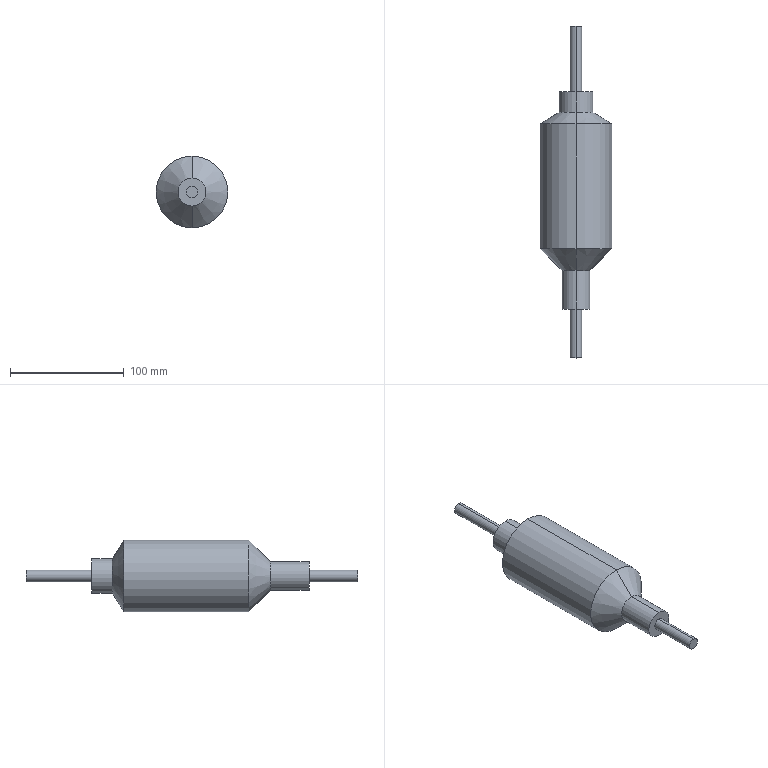Part | STEP file | Torque wrench | 1 solid | 18 faces | box 63.096 x 292.35 x 63.096 mm | volume 430044 mm3 | cylinder 10 | cone 4 | plane 4 | commonest cylinder face diameters 10.173 x4 24.731 x2 30 x2 63.096 x2
STEP:
#1=CARTESIAN_POINT('',(0.,0.,0.));
#2=DIRECTION('',(0.,0.,1.));
#3=DIRECTION('',(1.,0.,0.));
#4=AXIS2_PLACEMENT_3D('',#1,#2,#3);
#5=CARTESIAN_POINT('',(0.,-28.322,-31.548));
#6=VERTEX_POINT('',#5);
#7=CARTESIAN_POINT('',(0.,-28.322,31.548));
#8=VERTEX_POINT('',#7);
#9=CARTESIAN_POINT('',(0.,-28.322,0.));
#10=DIRECTION('',(0.,-1.,0.));
#11=DIRECTION('',(0.,0.,-1.));
#12=AXIS2_PLACEMENT_3D('',#9,#10,#11);
#13=CIRCLE('',#12,31.548);
#14=CARTESIAN_POINT('',(0.,-234.525,0.));
#15=DIRECTION('',(0.,-1.,0.));
#16=DIRECTION('',(0.,0.,-1.));
#17=AXIS2_PLACEMENT_3D('',#14,#15,#16);
#18=CYLINDRICAL_SURFACE('',#17,31.548);
#19=CARTESIAN_POINT('',(0.,-206.203));
#20=DIRECTION('',(1.,0.));
#21=VECTOR('',#20,1.);
#22=LINE('',#19,#21);
#23=(GEOMETRIC_REPRESENTATION_CONTEXT(2)PARAMETRIC_REPRESENTATION_CONTEXT()REPRESENTATION_CONTEXT('',''));
#24=DEFINITIONAL_REPRESENTATION('',(#22),#23);
#25=PCURVE('',#18,#24);
#26=CARTESIAN_POINT('',(0.,-28.322,0.));
#27=DIRECTION('',(0.,-1.,0.));
#28=DIRECTION('',(0.,0.,-1.));
#29=AXIS2_PLACEMENT_3D('',#26,#27,#28);
#30=CONICAL_SURFACE('',#29,31.548,1.025);
#31=CARTESIAN_POINT('',(0.,0.));
#32=DIRECTION('',(1.,0.));
#33=VECTOR('',#32,1.);
#34=LINE('',#31,#33);
#35=(GEOMETRIC_REPRESENTATION_CONTEXT(2)PARAMETRIC_REPRESENTATION_CONTEXT()REPRESENTATION_CONTEXT('',''));
#36=DEFINITIONAL_REPRESENTATION('',(#34),#35);
#37=PCURVE('',#30,#36);
#38=SURFACE_CURVE('',#13,(#25,#37),.PCURVE_S1.);
#39=EDGE_CURVE('',#6,#8,#38,.T.);
#40=ORIENTED_EDGE('',*,*,#39,.T.);
#41=CARTESIAN_POINT('',(0.,-138.276,31.548));
#42=VERTEX_POINT('',#41);
#43=CARTESIAN_POINT('',(0.,-234.525,31.548));
#44=DIRECTION('',(0.,-1.,0.));
#45=VECTOR('',#44,1.);
#46=LINE('',#43,#45);
#47=CARTESIAN_POINT('',(3.142,0.));
#48=DIRECTION('',(0.,1.));
#49=VECTOR('',#48,1.);
#50=LINE('',#47,#49);
#51=(GEOMETRIC_REPRESENTATION_CONTEXT(2)PARAMETRIC_REPRESENTATION_CONTEXT()REPRESENTATION_CONTEXT('',''));
#52=DEFINITIONAL_REPRESENTATION('',(#50),#51);
#53=PCURVE('',#18,#52);
#54=CARTESIAN_POINT('',(0.,-234.525,0.));
#55=DIRECTION('',(0.,-1.,0.));
#56=DIRECTION('',(0.,0.,-1.));
#57=AXIS2_PLACEMENT_3D('',#54,#55,#56);
#58=CYLINDRICAL_SURFACE('',#57,31.548);
#59=CARTESIAN_POINT('',(3.142,0.));
#60=DIRECTION('',(0.,1.));
#61=VECTOR('',#60,1.);
#62=LINE('',#59,#61);
#63=(GEOMETRIC_REPRESENTATION_CONTEXT(2)PARAMETRIC_REPRESENTATION_CONTEXT()REPRESENTATION_CONTEXT('',''));
#64=DEFINITIONAL_REPRESENTATION('',(#62),#63);
#65=PCURVE('',#58,#64);
#66=SURFACE_CURVE('',#46,(#53,#65),.PCURVE_S1.);
#67=EDGE_CURVE('',#8,#42,#66,.T.);
#68=ORIENTED_EDGE('',*,*,#67,.T.);
#69=CARTESIAN_POINT('',(0.,-138.276,-31.548));
#70=VERTEX_POINT('',#69);
#71=CARTESIAN_POINT('',(0.,-138.276,0.));
#72=DIRECTION('',(0.,1.,0.));
#73=DIRECTION('',(0.,0.,-1.));
#74=AXIS2_PLACEMENT_3D('',#71,#72,#73);
#75=CIRCLE('',#74,31.548);
#76=CARTESIAN_POINT('',(6.283,-96.249));
#77=DIRECTION('',(-1.,0.));
#78=VECTOR('',#77,1.);
#79=LINE('',#76,#78);
#80=(GEOMETRIC_REPRESENTATION_CONTEXT(2)PARAMETRIC_REPRESENTATION_CONTEXT()REPRESENTATION_CONTEXT('',''));
#81=DEFINITIONAL_REPRESENTATION('',(#79),#80);
#82=PCURVE('',#18,#81);
#83=CARTESIAN_POINT('',(0.,-138.276,0.));
#84=DIRECTION('',(0.,1.,0.));
#85=DIRECTION('',(0.,0.,1.));
#86=AXIS2_PLACEMENT_3D('',#83,#84,#85);
#87=CONICAL_SURFACE('',#86,31.548,0.7844);
#88=CARTESIAN_POINT('',(-3.142,0.));
#89=DIRECTION('',(1.,0.));
#90=VECTOR('',#89,1.);
#91=LINE('',#88,#90);
#92=(GEOMETRIC_REPRESENTATION_CONTEXT(2)PARAMETRIC_REPRESENTATION_CONTEXT()REPRESENTATION_CONTEXT('',''));
#93=DEFINITIONAL_REPRESENTATION('',(#91),#92);
#94=PCURVE('',#87,#93);
#95=SURFACE_CURVE('',#75,(#82,#94),.PCURVE_S1.);
#96=EDGE_CURVE('',#42,#70,#95,.T.);
#97=ORIENTED_EDGE('',*,*,#96,.T.);
#98=CARTESIAN_POINT('',(0.,-234.525,-31.548));
#99=DIRECTION('',(0.,-1.,0.));
#100=VECTOR('',#99,1.);
#101=LINE('',#98,#100);
#102=CARTESIAN_POINT('',(0.,0.));
#103=DIRECTION('',(0.,1.));
#104=VECTOR('',#103,1.);
#105=LINE('',#102,#104);
#106=(GEOMETRIC_REPRESENTATION_CONTEXT(2)PARAMETRIC_REPRESENTATION_CONTEXT()REPRESENTATION_CONTEXT('',''));
#107=DEFINITIONAL_REPRESENTATION('',(#105),#106);
#108=PCURVE('',#18,#107);
#109=CARTESIAN_POINT('',(6.283,0.));
#110=DIRECTION('',(0.,1.));
#111=VECTOR('',#110,1.);
#112=LINE('',#109,#111);
#113=(GEOMETRIC_REPRESENTATION_CONTEXT(2)PARAMETRIC_REPRESENTATION_CONTEXT()REPRESENTATION_CONTEXT('',''));
#114=DEFINITIONAL_REPRESENTATION('',(#112),#113);
#115=PCURVE('',#58,#114);
#116=SURFACE_CURVE('',#101,(#108,#115),.PCURVE_S1.);
#117=EDGE_CURVE('',#6,#70,#116,.T.);
#118=ORIENTED_EDGE('',*,*,#117,.F.);
#119=EDGE_LOOP('',(#40,#68,#97,#118));
#120=FACE_BOUND('',#119,.T.);
#121=ADVANCED_FACE('',(#120),#18,.T.);
#122=CARTESIAN_POINT('',(0.,-157.498,12.365));
#123=VERTEX_POINT('',#122);
#124=CARTESIAN_POINT('',(0.,-157.498,-12.365));
#125=VERTEX_POINT('',#124);
#126=CARTESIAN_POINT('',(0.,-157.498,0.));
#127=DIRECTION('',(0.,1.,0.));
#128=DIRECTION('',(0.,0.,1.));
#129=AXIS2_PLACEMENT_3D('',#126,#127,#128);
#130=CIRCLE('',#129,12.365);
#131=CARTESIAN_POINT('',(0.,-19.222));
#132=DIRECTION('',(1.,0.));
#133=VECTOR('',#132,1.);
#134=LINE('',#131,#133);
#135=(GEOMETRIC_REPRESENTATION_CONTEXT(2)PARAMETRIC_REPRESENTATION_CONTEXT()REPRESENTATION_CONTEXT('',''));
#136=DEFINITIONAL_REPRESENTATION('',(#134),#135);
#137=PCURVE('',#87,#136);
#138=CARTESIAN_POINT('',(0.,-234.525,0.));
#139=DIRECTION('',(0.,-1.,0.));
#140=DIRECTION('',(0.,0.,-1.));
#141=AXIS2_PLACEMENT_3D('',#138,#139,#140);
#142=CYLINDRICAL_SURFACE('',#141,12.365);
#143=CARTESIAN_POINT('',(3.142,-77.027));
#144=DIRECTION('',(-1.,0.));
#145=VECTOR('',#144,1.);
#146=LINE('',#143,#145);
#147=(GEOMETRIC_REPRESENTATION_CONTEXT(2)PARAMETRIC_REPRESENTATION_CONTEXT()REPRESENTATION_CONTEXT('',''));
#148=DEFINITIONAL_REPRESENTATION('',(#146),#147);
#149=PCURVE('',#142,#148);
#150=SURFACE_CURVE('',#130,(#137,#149),.PCURVE_S1.);
#151=EDGE_CURVE('',#123,#125,#150,.T.);
#152=ORIENTED_EDGE('',*,*,#151,.T.);
#153=CARTESIAN_POINT('',(0.,-138.276,-31.548));
#154=DIRECTION('',(0.,0.7078,-0.7064));
#155=VECTOR('',#154,1.);
#156=LINE('',#153,#155);
#157=CARTESIAN_POINT('',(3.142,0.));
#158=DIRECTION('',(0.,1.));
#159=VECTOR('',#158,1.);
#160=LINE('',#157,#159);
#161=(GEOMETRIC_REPRESENTATION_CONTEXT(2)PARAMETRIC_REPRESENTATION_CONTEXT()REPRESENTATION_CONTEXT('',''));
#162=DEFINITIONAL_REPRESENTATION('',(#160),#161);
#163=PCURVE('',#87,#162);
#164=CARTESIAN_POINT('',(0.,-138.276,0.));
#165=DIRECTION('',(0.,1.,0.));
#166=DIRECTION('',(0.,0.,1.));
#167=AXIS2_PLACEMENT_3D('',#164,#165,#166);
#168=CONICAL_SURFACE('',#167,31.548,0.7844);
#169=CARTESIAN_POINT('',(3.142,0.));
#170=DIRECTION('',(0.,1.));
#171=VECTOR('',#170,1.);
#172=LINE('',#169,#171);
#173=(GEOMETRIC_REPRESENTATION_CONTEXT(2)PARAMETRIC_REPRESENTATION_CONTEXT()REPRESENTATION_CONTEXT('',''));
#174=DEFINITIONAL_REPRESENTATION('',(#172),#173);
#175=PCURVE('',#168,#174);
#176=SURFACE_CURVE('',#156,(#163,#175),.PCURVE_S1.);
#177=EDGE_CURVE('',#125,#70,#176,.T.);
#178=ORIENTED_EDGE('',*,*,#177,.T.);
#179=ORIENTED_EDGE('',*,*,#96,.F.);
#180=CARTESIAN_POINT('',(0.,-138.276,31.548));
#181=DIRECTION('',(0.,0.7078,0.7064));
#182=VECTOR('',#181,1.);
#183=LINE('',#180,#182);
#184=CARTESIAN_POINT('',(0.,0.));
#185=DIRECTION('',(0.,1.));
#186=VECTOR('',#185,1.);
#187=LINE('',#184,#186);
#188=(GEOMETRIC_REPRESENTATION_CONTEXT(2)PARAMETRIC_REPRESENTATION_CONTEXT()REPRESENTATION_CONTEXT('',''));
#189=DEFINITIONAL_REPRESENTATION('',(#187),#188);
#190=PCURVE('',#87,#189);
#191=CARTESIAN_POINT('',(6.283,0.));
#192=DIRECTION('',(0.,1.));
#193=VECTOR('',#192,1.);
#194=LINE('',#191,#193);
#195=(GEOMETRIC_REPRESENTATION_CONTEXT(2)PARAMETRIC_REPRESENTATION_CONTEXT()REPRESENTATION_CONTEXT('',''));
#196=DEFINITIONAL_REPRESENTATION('',(#194),#195);
#197=PCURVE('',#168,#196);
#198=SURFACE_CURVE('',#183,(#190,#197),.PCURVE_S1.);
#199=EDGE_CURVE('',#123,#42,#198,.T.);
#200=ORIENTED_EDGE('',*,*,#199,.F.);
#201=EDGE_LOOP('',(#152,#178,#179,#200));
#202=FACE_BOUND('',#201,.T.);
#203=ADVANCED_FACE('',(#202),#87,.T.);
#204=CARTESIAN_POINT('',(0.,-18.263,-15.));
#205=VERTEX_POINT('',#204);
#206=CARTESIAN_POINT('',(0.,-18.263,15.));
#207=VERTEX_POINT('',#206);
#208=CARTESIAN_POINT('',(0.,-18.263,0.));
#209=DIRECTION('',(0.,-1.,0.));
#210=DIRECTION('',(0.,0.,-1.));
#211=AXIS2_PLACEMENT_3D('',#208,#209,#210);
#212=CIRCLE('',#211,15.);
#213=CARTESIAN_POINT('',(0.,-10.059));
#214=DIRECTION('',(1.,0.));
#215=VECTOR('',#214,1.);
#216=LINE('',#213,#215);
#217=(GEOMETRIC_REPRESENTATION_CONTEXT(2)PARAMETRIC_REPRESENTATION_CONTEXT()REPRESENTATION_CONTEXT('',''));
#218=DEFINITIONAL_REPRESENTATION('',(#216),#217);
#219=PCURVE('',#30,#218);
#220=CARTESIAN_POINT('',(0.,-234.525,0.));
#221=DIRECTION('',(0.,-1.,0.));
#222=DIRECTION('',(0.,0.,-1.));
#223=AXIS2_PLACEMENT_3D('',#220,#221,#222);
#224=CYLINDRICAL_SURFACE('',#223,15.);
#225=CARTESIAN_POINT('',(0.,-216.262));
#226=DIRECTION('',(1.,0.));
#227=VECTOR('',#226,1.);
#228=LINE('',#225,#227);
#229=(GEOMETRIC_REPRESENTATION_CONTEXT(2)PARAMETRIC_REPRESENTATION_CONTEXT()REPRESENTATION_CONTEXT('',''));
#230=DEFINITIONAL_REPRESENTATION('',(#228),#229);
#231=PCURVE('',#224,#230);
#232=SURFACE_CURVE('',#212,(#219,#231),.PCURVE_S1.);
#233=EDGE_CURVE('',#205,#207,#232,.T.);
#234=ORIENTED_EDGE('',*,*,#233,.T.);
#235=CARTESIAN_POINT('',(0.,-28.322,31.548));
#236=DIRECTION('',(0.,-0.5194,0.8545));
#237=VECTOR('',#236,1.);
#238=LINE('',#235,#237);
#239=CARTESIAN_POINT('',(3.142,0.));
#240=DIRECTION('',(0.,1.));
#241=VECTOR('',#240,1.);
#242=LINE('',#239,#241);
#243=(GEOMETRIC_REPRESENTATION_CONTEXT(2)PARAMETRIC_REPRESENTATION_CONTEXT()REPRESENTATION_CONTEXT('',''));
#244=DEFINITIONAL_REPRESENTATION('',(#242),#243);
#245=PCURVE('',#30,#244);
#246=CARTESIAN_POINT('',(0.,-28.322,0.));
#247=DIRECTION('',(0.,-1.,0.));
#248=DIRECTION('',(0.,0.,-1.));
#249=AXIS2_PLACEMENT_3D('',#246,#247,#248);
#250=CONICAL_SURFACE('',#249,31.548,1.025);
#251=CARTESIAN_POINT('',(3.142,0.));
#252=DIRECTION('',(0.,1.));
#253=VECTOR('',#252,1.);
#254=LINE('',#251,#253);
#255=(GEOMETRIC_REPRESENTATION_CONTEXT(2)PARAMETRIC_REPRESENTATION_CONTEXT()REPRESENTATION_CONTEXT('',''));
#256=DEFINITIONAL_REPRESENTATION('',(#254),#255);
#257=PCURVE('',#250,#256);
#258=SURFACE_CURVE('',#238,(#245,#257),.PCURVE_S1.);
#259=EDGE_CURVE('',#207,#8,#258,.T.);
#260=ORIENTED_EDGE('',*,*,#259,.T.);
#261=ORIENTED_EDGE('',*,*,#39,.F.);
#262=CARTESIAN_POINT('',(0.,-28.322,-31.548));
#263=DIRECTION('',(0.,-0.5194,-0.8545));
#264=VECTOR('',#263,1.);
#265=LINE('',#262,#264);
#266=CARTESIAN_POINT('',(0.,0.));
#267=DIRECTION('',(0.,1.));
#268=VECTOR('',#267,1.);
#269=LINE('',#266,#268);
#270=(GEOMETRIC_REPRESENTATION_CONTEXT(2)PARAMETRIC_REPRESENTATION_CONTEXT()REPRESENTATION_CONTEXT('',''));
#271=DEFINITIONAL_REPRESENTATION('',(#269),#270);
#272=PCURVE('',#30,#271);
#273=CARTESIAN_POINT('',(6.283,0.));
#274=DIRECTION('',(0.,1.));
#275=VECTOR('',#274,1.);
#276=LINE('',#273,#275);
#277=(GEOMETRIC_REPRESENTATION_CONTEXT(2)PARAMETRIC_REPRESENTATION_CONTEXT()REPRESENTATION_CONTEXT('',''));
#278=DEFINITIONAL_REPRESENTATION('',(#276),#277);
#279=PCURVE('',#250,#278);
#280=SURFACE_CURVE('',#265,(#272,#279),.PCURVE_S1.);
#281=EDGE_CURVE('',#205,#6,#280,.T.);
#282=ORIENTED_EDGE('',*,*,#281,.F.);
#283=EDGE_LOOP('',(#234,#260,#261,#282));
#284=FACE_BOUND('',#283,.T.);
#285=ADVANCED_FACE('',(#284),#30,.T.);
#286=ORIENTED_EDGE('',*,*,#151,.F.);
#287=CARTESIAN_POINT('',(0.,-191.509,12.365));
#288=VERTEX_POINT('',#287);
#289=CARTESIAN_POINT('',(0.,-234.525,12.365));
#290=DIRECTION('',(0.,-1.,0.));
#291=VECTOR('',#290,1.);
#292=LINE('',#289,#291);
#293=CARTESIAN_POINT('',(3.142,0.));
#294=DIRECTION('',(0.,1.));
#295=VECTOR('',#294,1.);
#296=LINE('',#293,#295);
#297=(GEOMETRIC_REPRESENTATION_CONTEXT(2)PARAMETRIC_REPRESENTATION_CONTEXT()REPRESENTATION_CONTEXT('',''));
#298=DEFINITIONAL_REPRESENTATION('',(#296),#297);
#299=PCURVE('',#142,#298);
#300=CARTESIAN_POINT('',(0.,-234.525,0.));
#301=DIRECTION('',(0.,-1.,0.));
#302=DIRECTION('',(0.,0.,-1.));
#303=AXIS2_PLACEMENT_3D('',#300,#301,#302);
#304=CYLINDRICAL_SURFACE('',#303,12.365);
#305=CARTESIAN_POINT('',(3.142,0.));
#306=DIRECTION('',(0.,1.));
#307=VECTOR('',#306,1.);
#308=LINE('',#305,#307);
#309=(GEOMETRIC_REPRESENTATION_CONTEXT(2)PARAMETRIC_REPRESENTATION_CONTEXT()REPRESENTATION_CONTEXT('',''));
#310=DEFINITIONAL_REPRESENTATION('',(#308),#309);
#311=PCURVE('',#304,#310);
#312=SURFACE_CURVE('',#292,(#299,#311),.PCURVE_S1.);
#313=EDGE_CURVE('',#123,#288,#312,.T.);
#314=ORIENTED_EDGE('',*,*,#313,.T.);
#315=CARTESIAN_POINT('',(0.,-191.509,-12.365));
#316=VERTEX_POINT('',#315);
#317=CARTESIAN_POINT('',(0.,-191.509,0.));
#318=DIRECTION('',(0.,1.,0.));
#319=DIRECTION('',(0.,0.,-1.));
#320=AXIS2_PLACEMENT_3D('',#317,#318,#319);
#321=CIRCLE('',#320,12.365);
#322=CARTESIAN_POINT('',(6.283,-43.016));
#323=DIRECTION('',(-1.,0.));
#324=VECTOR('',#323,1.);
#325=LINE('',#322,#324);
#326=(GEOMETRIC_REPRESENTATION_CONTEXT(2)PARAMETRIC_REPRESENTATION_CONTEXT()REPRESENTATION_CONTEXT('',''));
#327=DEFINITIONAL_REPRESENTATION('',(#325),#326);
#328=PCURVE('',#142,#327);
#329=CARTESIAN_POINT('',(12.365,-191.509,0.));
#330=DIRECTION('',(0.,-1.,0.));
#331=DIRECTION('',(0.,0.,-1.));
#332=AXIS2_PLACEMENT_3D('',#329,#330,#331);
#333=PLANE('',#332);
#334=CARTESIAN_POINT('',(12.365,-12.365));
#335=CARTESIAN_POINT('',(12.365,-33.783));
#336=CARTESIAN_POINT('',(-6.183,-23.074));
#337=CARTESIAN_POINT('',(-24.731,-12.365));
#338=CARTESIAN_POINT('',(-6.183,-1.657));
#339=CARTESIAN_POINT('',(12.365,9.052));
#340=CARTESIAN_POINT('',(12.365,-12.365));
#341=(BOUNDED_CURVE()B_SPLINE_CURVE(2,(#334,#335,#336,#337,#338,#339,#340),.UNSPECIFIED.,.T.,.F.)B_SPLINE_CURVE_WITH_KNOTS((1,2,2,2,2,1),(-2.094,0.,2.094,4.189,6.283,8.378),.UNSPECIFIED.)CURVE()GEOMETRIC_REPRESENTATION_ITEM()RATIONAL_B_SPLINE_CURVE((1.,0.5,1.,0.5,1.,0.5,1.))REPRESENTATION_ITEM(''));
#342=(GEOMETRIC_REPRESENTATION_CONTEXT(2)PARAMETRIC_REPRESENTATION_CONTEXT()REPRESENTATION_CONTEXT('',''));
#343=DEFINITIONAL_REPRESENTATION('',(#341),#342);
#344=PCURVE('',#333,#343);
#345=SURFACE_CURVE('',#321,(#328,#344),.PCURVE_S1.);
#346=EDGE_CURVE('',#288,#316,#345,.T.);
#347=ORIENTED_EDGE('',*,*,#346,.T.);
#348=CARTESIAN_POINT('',(0.,-234.525,-12.365));
#349=DIRECTION('',(0.,-1.,0.));
#350=VECTOR('',#349,1.);
#351=LINE('',#348,#350);
#352=CARTESIAN_POINT('',(0.,0.));
#353=DIRECTION('',(0.,1.));
#354=VECTOR('',#353,1.);
#355=LINE('',#352,#354);
#356=(GEOMETRIC_REPRESENTATION_CONTEXT(2)PARAMETRIC_REPRESENTATION_CONTEXT()REPRESENTATION_CONTEXT('',''));
#357=DEFINITIONAL_REPRESENTATION('',(#355),#356);
#358=PCURVE('',#142,#357);
#359=CARTESIAN_POINT('',(6.283,0.));
#360=DIRECTION('',(0.,1.));
#361=VECTOR('',#360,1.);
#362=LINE('',#359,#361);
#363=(GEOMETRIC_REPRESENTATION_CONTEXT(2)PARAMETRIC_REPRESENTATION_CONTEXT()REPRESENTATION_CONTEXT('',''));
#364=DEFINITIONAL_REPRESENTATION('',(#362),#363);
#365=PCURVE('',#304,#364);
#366=SURFACE_CURVE('',#351,(#358,#365),.PCURVE_S1.);
#367=EDGE_CURVE('',#125,#316,#366,.T.);
#368=ORIENTED_EDGE('',*,*,#367,.F.);
#369=EDGE_LOOP('',(#286,#314,#347,#368));
#370=FACE_BOUND('',#369,.T.);
#371=ADVANCED_FACE('',(#370),#142,.T.);
#372=CARTESIAN_POINT('',(0.,0.,-15.));
#373=VERTEX_POINT('',#372);
#374=CARTESIAN_POINT('',(0.,0.,15.));
#375=VERTEX_POINT('',#374);
#376=CARTESIAN_POINT('',(0.,0.,0.));
#377=DIRECTION('',(0.,-1.,0.));
#378=DIRECTION('',(0.,0.,-1.));
#379=AXIS2_PLACEMENT_3D('',#376,#377,#378);
#380=CIRCLE('',#379,15.);
#381=CARTESIAN_POINT('',(0.,-234.525));
#382=DIRECTION('',(1.,0.));
#383=VECTOR('',#382,1.);
#384=LINE('',#381,#383);
#385=(GEOMETRIC_REPRESENTATION_CONTEXT(2)PARAMETRIC_REPRESENTATION_CONTEXT()REPRESENTATION_CONTEXT('',''));
#386=DEFINITIONAL_REPRESENTATION('',(#384),#385);
#387=PCURVE('',#224,#386);
#388=CARTESIAN_POINT('',(5.086,0.,0.));
#389=DIRECTION('',(0.,1.,0.));
#390=DIRECTION('',(0.,0.,1.));
#391=AXIS2_PLACEMENT_3D('',#388,#389,#390);
#392=PLANE('',#391);
#393=CARTESIAN_POINT('',(-15.,-5.086));
#394=CARTESIAN_POINT('',(-15.,20.894));
#395=CARTESIAN_POINT('',(7.5,7.904));
#396=CARTESIAN_POINT('',(30.,-5.086));
#397=CARTESIAN_POINT('',(7.5,-18.077));
#398=CARTESIAN_POINT('',(-15.,-31.067));
#399=CARTESIAN_POINT('',(-15.,-5.086));
#400=(BOUNDED_CURVE()B_SPLINE_CURVE(2,(#393,#394,#395,#396,#397,#398,#399),.UNSPECIFIED.,.T.,.F.)B_SPLINE_CURVE_WITH_KNOTS((1,2,2,2,2,1),(-2.094,0.,2.094,4.189,6.283,8.378),.UNSPECIFIED.)CURVE()GEOMETRIC_REPRESENTATION_ITEM()RATIONAL_B_SPLINE_CURVE((1.,0.5,1.,0.5,1.,0.5,1.))REPRESENTATION_ITEM(''));
#401=(GEOMETRIC_REPRESENTATION_CONTEXT(2)PARAMETRIC_REPRESENTATION_CONTEXT()REPRESENTATION_CONTEXT('',''));
#402=DEFINITIONAL_REPRESENTATION('',(#400),#401);
#403=PCURVE('',#392,#402);
#404=SURFACE_CURVE('',#380,(#387,#403),.PCURVE_S1.);
#405=EDGE_CURVE('',#373,#375,#404,.T.);
#406=ORIENTED_EDGE('',*,*,#405,.T.);
#407=CARTESIAN_POINT('',(0.,-234.525,15.));
#408=DIRECTION('',(0.,-1.,0.));
#409=VECTOR('',#408,1.);
#410=LINE('',#407,#409);
#411=CARTESIAN_POINT('',(3.142,0.));
#412=DIRECTION('',(0.,1.));
#413=VECTOR('',#412,1.);
#414=LINE('',#411,#413);
#415=(GEOMETRIC_REPRESENTATION_CONTEXT(2)PARAMETRIC_REPRESENTATION_CONTEXT()REPRESENTATION_CONTEXT('',''));
#416=DEFINITIONAL_REPRESENTATION('',(#414),#415);
#417=PCURVE('',#224,#416);
#418=CARTESIAN_POINT('',(0.,-234.525,0.));
#419=DIRECTION('',(0.,-1.,0.));
#420=DIRECTION('',(0.,0.,-1.));
#421=AXIS2_PLACEMENT_3D('',#418,#419,#420);
#422=CYLINDRICAL_SURFACE('',#421,15.);
#423=CARTESIAN_POINT('',(3.142,0.));
#424=DIRECTION('',(0.,1.));
#425=VECTOR('',#424,1.);
#426=LINE('',#423,#425);
#427=(GEOMETRIC_REPRESENTATION_CONTEXT(2)PARAMETRIC_REPRESENTATION_CONTEXT()REPRESENTATION_CONTEXT('',''));
#428=DEFINITIONAL_REPRESENTATION('',(#426),#427);
#429=PCURVE('',#422,#428);
#430=SURFACE_CURVE('',#410,(#417,#429),.PCURVE_S1.);
#431=EDGE_CURVE('',#375,#207,#430,.T.);
#432=ORIENTED_EDGE('',*,*,#431,.T.);
#433=ORIENTED_EDGE('',*,*,#233,.F.);
#434=CARTESIAN_POINT('',(0.,-234.525,-15.));
#435=DIRECTION('',(0.,-1.,0.));
#436=VECTOR('',#435,1.);
#437=LINE('',#434,#436);
#438=CARTESIAN_POINT('',(0.,0.));
#439=DIRECTION('',(0.,1.));
#440=VECTOR('',#439,1.);
#441=LINE('',#438,#440);
#442=(GEOMETRIC_REPRESENTATION_CONTEXT(2)PARAMETRIC_REPRESENTATION_CONTEXT()REPRESENTATION_CONTEXT('',''));
#443=DEFINITIONAL_REPRESENTATION('',(#441),#442);
#444=PCURVE('',#224,#443);
#445=CARTESIAN_POINT('',(6.283,0.));
#446=DIRECTION('',(0.,1.));
#447=VECTOR('',#446,1.);
#448=LINE('',#445,#447);
#449=(GEOMETRIC_REPRESENTATION_CONTEXT(2)PARAMETRIC_REPRESENTATION_CONTEXT()REPRESENTATION_CONTEXT('',''));
#450=DEFINITIONAL_REPRESENTATION('',(#448),#449);
#451=PCURVE('',#422,#450);
#452=SURFACE_CURVE('',#437,(#444,#451),.PCURVE_S1.);
#453=EDGE_CURVE('',#373,#205,#452,.T.);
#454=ORIENTED_EDGE('',*,*,#453,.F.);
#455=EDGE_LOOP('',(#406,#432,#433,#454));
#456=FACE_BOUND('',#455,.T.);
#457=ADVANCED_FACE('',(#456),#224,.T.);
#458=CARTESIAN_POINT('',(0.,-191.509,5.086));
#459=VERTEX_POINT('',#458);
#460=CARTESIAN_POINT('',(0.,-191.509,-5.086));
#461=VERTEX_POINT('',#460);
#462=CARTESIAN_POINT('',(0.,-191.509,0.));
#463=DIRECTION('',(0.,1.,0.));
#464=DIRECTION('',(0.,0.,-1.));
#465=AXIS2_PLACEMENT_3D('',#462,#463,#464);
#466=CIRCLE('',#465,5.086);
#467=CARTESIAN_POINT('',(0.,-234.525,0.));
#468=DIRECTION('',(0.,-1.,0.));
#469=DIRECTION('',(0.,0.,-1.));
#470=AXIS2_PLACEMENT_3D('',#467,#468,#469);
#471=CYLINDRICAL_SURFACE('',#470,5.086);
#472=CARTESIAN_POINT('',(6.283,-43.016));
#473=DIRECTION('',(-1.,0.));
#474=VECTOR('',#473,1.);
#475=LINE('',#472,#474);
#476=(GEOMETRIC_REPRESENTATION_CONTEXT(2)PARAMETRIC_REPRESENTATION_CONTEXT()REPRESENTATION_CONTEXT('',''));
#477=DEFINITIONAL_REPRESENTATION('',(#475),#476);
#478=PCURVE('',#471,#477);
#479=CARTESIAN_POINT('',(5.086,-12.365));
#480=CARTESIAN_POINT('',(5.086,-21.175));
#481=CARTESIAN_POINT('',(-2.543,-16.77));
#482=CARTESIAN_POINT('',(-10.173,-12.365));
#483=CARTESIAN_POINT('',(-2.543,-7.96));
#484=CARTESIAN_POINT('',(5.086,-3.555));
#485=CARTESIAN_POINT('',(5.086,-12.365));
#486=(BOUNDED_CURVE()B_SPLINE_CURVE(2,(#479,#480,#481,#482,#483,#484,#485),.UNSPECIFIED.,.T.,.F.)B_SPLINE_CURVE_WITH_KNOTS((1,2,2,2,2,1),(-2.094,0.,2.094,4.189,6.283,8.378),.UNSPECIFIED.)CURVE()GEOMETRIC_REPRESENTATION_ITEM()RATIONAL_B_SPLINE_CURVE((1.,0.5,1.,0.5,1.,0.5,1.))REPRESENTATION_ITEM(''));
#487=(GEOMETRIC_REPRESENTATION_CONTEXT(2)PARAMETRIC_REPRESENTATION_CONTEXT()REPRESENTATION_CONTEXT('',''));
#488=DEFINITIONAL_REPRESENTATION('',(#486),#487);
#489=PCURVE('',#333,#488);
#490=SURFACE_CURVE('',#466,(#478,#489),.PCURVE_S1.);
#491=EDGE_CURVE('',#459,#461,#490,.T.);
#492=ORIENTED_EDGE('',*,*,#491,.F.);
#493=CARTESIAN_POINT('',(0.,-234.525,5.086));
#494=VERTEX_POINT('',#493);
#495=CARTESIAN_POINT('',(0.,-234.525,5.086));
#496=DIRECTION('',(0.,-1.,0.));
#497=VECTOR('',#496,1.);
#498=LINE('',#495,#497);
#499=CARTESIAN_POINT('',(3.142,0.));
#500=DIRECTION('',(0.,1.));
#501=VECTOR('',#500,1.);
#502=LINE('',#499,#501);
#503=(GEOMETRIC_REPRESENTATION_CONTEXT(2)PARAMETRIC_REPRESENTATION_CONTEXT()REPRESENTATION_CONTEXT('',''));
#504=DEFINITIONAL_REPRESENTATION('',(#502),#503);
#505=PCURVE('',#471,#504);
#506=CARTESIAN_POINT('',(0.,-234.525,0.));
#507=DIRECTION('',(0.,-1.,0.));
#508=DIRECTION('',(0.,0.,-1.));
#509=AXIS2_PLACEMENT_3D('',#506,#507,#508);
#510=CYLINDRICAL_SURFACE('',#509,5.086);
#511=CARTESIAN_POINT('',(3.142,0.));
#512=DIRECTION('',(0.,1.));
#513=VECTOR('',#512,1.);
#514=LINE('',#511,#513);
#515=(GEOMETRIC_REPRESENTATION_CONTEXT(2)PARAMETRIC_REPRESENTATION_CONTEXT()REPRESENTATION_CONTEXT('',''));
#516=DEFINITIONAL_REPRESENTATION('',(#514),#515);
#517=PCURVE('',#510,#516);
#518=SURFACE_CURVE('',#498,(#505,#517),.PCURVE_S1.);
#519=EDGE_CURVE('',#459,#494,#518,.T.);
#520=ORIENTED_EDGE('',*,*,#519,.T.);
#521=CARTESIAN_POINT('',(0.,-234.525,-5.086));
#522=VERTEX_POINT('',#521);
#523=CARTESIAN_POINT('',(0.,-234.525,0.));
#524=DIRECTION('',(0.,1.,0.));
#525=DIRECTION('',(0.,0.,-1.));
#526=AXIS2_PLACEMENT_3D('',#523,#524,#525);
#527=CIRCLE('',#526,5.086);
#528=CARTESIAN_POINT('',(6.283,0.));
#529=DIRECTION('',(-1.,0.));
#530=VECTOR('',#529,1.);
#531=LINE('',#528,#530);
#532=(GEOMETRIC_REPRESENTATION_CONTEXT(2)PARAMETRIC_REPRESENTATION_CONTEXT()REPRESENTATION_CONTEXT('',''));
#533=DEFINITIONAL_REPRESENTATION('',(#531),#532);
#534=PCURVE('',#471,#533);
#535=CARTESIAN_POINT('',(5.086,-234.525,0.));
#536=DIRECTION('',(0.,-1.,0.));
#537=DIRECTION('',(0.,0.,-1.));
#538=AXIS2_PLACEMENT_3D('',#535,#536,#537);
#539=PLANE('',#538);
#540=CARTESIAN_POINT('',(5.086,-5.086));
#541=CARTESIAN_POINT('',(5.086,-13.896));
#542=CARTESIAN_POINT('',(-2.543,-9.491));
#543=CARTESIAN_POINT('',(-10.173,-5.086));
#544=CARTESIAN_POINT('',(-2.543,-0.6815));
#545=CARTESIAN_POINT('',(5.086,3.724));
#546=CARTESIAN_POINT('',(5.086,-5.086));
#547=(BOUNDED_CURVE()B_SPLINE_CURVE(2,(#540,#541,#542,#543,#544,#545,#546),.UNSPECIFIED.,.T.,.F.)B_SPLINE_CURVE_WITH_KNOTS((1,2,2,2,2,1),(-2.094,0.,2.094,4.189,6.283,8.378),.UNSPECIFIED.)CURVE()GEOMETRIC_REPRESENTATION_ITEM()RATIONAL_B_SPLINE_CURVE((1.,0.5,1.,0.5,1.,0.5,1.))REPRESENTATION_ITEM(''));
#548=(GEOMETRIC_REPRESENTATION_CONTEXT(2)PARAMETRIC_REPRESENTATION_CONTEXT()REPRESENTATION_CONTEXT('',''));
#549=DEFINITIONAL_REPRESENTATION('',(#547),#548);
#550=PCURVE('',#539,#549);
#551=SURFACE_CURVE('',#527,(#534,#550),.PCURVE_S1.);
#552=EDGE_CURVE('',#494,#522,#551,.T.);
#553=ORIENTED_EDGE('',*,*,#552,.T.);
#554=CARTESIAN_POINT('',(0.,-234.525,-5.086));
#555=DIRECTION('',(0.,-1.,0.));
#556=VECTOR('',#555,1.);
#557=LINE('',#554,#556);
#558=CARTESIAN_POINT('',(0.,0.));
#559=DIRECTION('',(0.,1.));
#560=VECTOR('',#559,1.);
#561=LINE('',#558,#560);
#562=(GEOMETRIC_REPRESENTATION_CONTEXT(2)PARAMETRIC_REPRESENTATION_CONTEXT()REPRESENTATION_CONTEXT('',''));
#563=DEFINITIONAL_REPRESENTATION('',(#561),#562);
#564=PCURVE('',#471,#563);
#565=CARTESIAN_POINT('',(6.283,0.));
#566=DIRECTION('',(0.,1.));
#567=VECTOR('',#566,1.);
#568=LINE('',#565,#567);
#569=(GEOMETRIC_REPRESENTATION_CONTEXT(2)PARAMETRIC_REPRESENTATION_CONTEXT()REPRESENTATION_CONTEXT('',''));
#570=DEFINITIONAL_REPRESENTATION('',(#568),#569);
#571=PCURVE('',#510,#570);
#572=SURFACE_CURVE('',#557,(#564,#571),.PCURVE_S1.);
#573=EDGE_CURVE('',#461,#522,#572,.T.);
#574=ORIENTED_EDGE('',*,*,#573,.F.);
#575=EDGE_LOOP('',(#492,#520,#553,#574));
#576=FACE_BOUND('',#575,.T.);
#577=ADVANCED_FACE('',(#576),#471,.T.);
#578=CARTESIAN_POINT('',(0.,57.825,-5.086));
#579=VERTEX_POINT('',#578);
#580=CARTESIAN_POINT('',(0.,57.825,5.086));
#581=VERTEX_POINT('',#580);
#582=CARTESIAN_POINT('',(0.,57.825,0.));
#583=DIRECTION('',(0.,-1.,0.));
#584=DIRECTION('',(0.,0.,-1.));
#585=AXIS2_PLACEMENT_3D('',#582,#583,#584);
#586=CIRCLE('',#585,5.086);
#587=CARTESIAN_POINT('',(0.,-234.525,0.));
#588=DIRECTION('',(0.,-1.,0.));
#589=DIRECTION('',(0.,0.,-1.));
#590=AXIS2_PLACEMENT_3D('',#587,#588,#589);
#591=CYLINDRICAL_SURFACE('',#590,5.086);
#592=CARTESIAN_POINT('',(0.,-292.35));
#593=DIRECTION('',(1.,0.));
#594=VECTOR('',#593,1.);
#595=LINE('',#592,#594);
#596=(GEOMETRIC_REPRESENTATION_CONTEXT(2)PARAMETRIC_REPRESENTATION_CONTEXT()REPRESENTATION_CONTEXT('',''));
#597=DEFINITIONAL_REPRESENTATION('',(#595),#596);
#598=PCURVE('',#591,#597);
#599=CARTESIAN_POINT('',(5.086,57.825,0.));
#600=DIRECTION('',(0.,1.,0.));
#601=DIRECTION('',(0.,0.,1.));
#602=AXIS2_PLACEMENT_3D('',#599,#600,#601);
#603=PLANE('',#602);
#604=CARTESIAN_POINT('',(-5.086,-5.086));
#605=CARTESIAN_POINT('',(-5.086,3.724));
#606=CARTESIAN_POINT('',(2.543,-0.6815));
#607=CARTESIAN_POINT('',(10.173,-5.086));
#608=CARTESIAN_POINT('',(2.543,-9.491));
#609=CARTESIAN_POINT('',(-5.086,-13.896));
#610=CARTESIAN_POINT('',(-5.086,-5.086));
#611=(BOUNDED_CURVE()B_SPLINE_CURVE(2,(#604,#605,#606,#607,#608,#609,#610),.UNSPECIFIED.,.T.,.F.)B_SPLINE_CURVE_WITH_KNOTS((1,2,2,2,2,1),(-2.094,0.,2.094,4.189,6.283,8.378),.UNSPECIFIED.)CURVE()GEOMETRIC_REPRESENTATION_ITEM()RATIONAL_B_SPLINE_CURVE((1.,0.5,1.,0.5,1.,0.5,1.))REPRESENTATION_ITEM(''));
#612=(GEOMETRIC_REPRESENTATION_CONTEXT(2)PARAMETRIC_REPRESENTATION_CONTEXT()REPRESENTATION_CONTEXT('',''));
#613=DEFINITIONAL_REPRESENTATION('',(#611),#612);
#614=PCURVE('',#603,#613);
#615=SURFACE_CURVE('',#586,(#598,#614),.PCURVE_S1.);
#616=EDGE_CURVE('',#579,#581,#615,.T.);
#617=ORIENTED_EDGE('',*,*,#616,.T.);
#618=CARTESIAN_POINT('',(0.,0.,5.086));
#619=VERTEX_POINT('',#618);
#620=CARTESIAN_POINT('',(0.,-234.525,5.086));
#621=DIRECTION('',(0.,-1.,0.));
#622=VECTOR('',#621,1.);
#623=LINE('',#620,#622);
#624=CARTESIAN_POINT('',(3.142,0.));
#625=DIRECTION('',(0.,1.));
#626=VECTOR('',#625,1.);
#627=LINE('',#624,#626);
#628=(GEOMETRIC_REPRESENTATION_CONTEXT(2)PARAMETRIC_REPRESENTATION_CONTEXT()REPRESENTATION_CONTEXT('',''));
#629=DEFINITIONAL_REPRESENTATION('',(#627),#628);
#630=PCURVE('',#591,#629);
#631=CARTESIAN_POINT('',(0.,-234.525,0.));
#632=DIRECTION('',(0.,-1.,0.));
#633=DIRECTION('',(0.,0.,-1.));
#634=AXIS2_PLACEMENT_3D('',#631,#632,#633);
#635=CYLINDRICAL_SURFACE('',#634,5.086);
#636=CARTESIAN_POINT('',(3.142,0.));
#637=DIRECTION('',(0.,1.));
#638=VECTOR('',#637,1.);
#639=LINE('',#636,#638);
#640=(GEOMETRIC_REPRESENTATION_CONTEXT(2)PARAMETRIC_REPRESENTATION_CONTEXT()REPRESENTATION_CONTEXT('',''));
#641=DEFINITIONAL_REPRESENTATION('',(#639),#640);
#642=PCURVE('',#635,#641);
#643=SURFACE_CURVE('',#623,(#630,#642),.PCURVE_S1.);
#644=EDGE_CURVE('',#581,#619,#643,.T.);
#645=ORIENTED_EDGE('',*,*,#644,.T.);
#646=CARTESIAN_POINT('',(0.,0.,-5.086));
#647=VERTEX_POINT('',#646);
#648=CARTESIAN_POINT('',(0.,0.,0.));
#649=DIRECTION('',(0.,-1.,0.));
#650=DIRECTION('',(0.,0.,-1.));
#651=AXIS2_PLACEMENT_3D('',#648,#649,#650);
#652=CIRCLE('',#651,5.086);
#653=CARTESIAN_POINT('',(0.,-234.525));
#654=DIRECTION('',(1.,0.));
#655=VECTOR('',#654,1.);
#656=LINE('',#653,#655);
#657=(GEOMETRIC_REPRESENTATION_CONTEXT(2)PARAMETRIC_REPRESENTATION_CONTEXT()REPRESENTATION_CONTEXT('',''));
#658=DEFINITIONAL_REPRESENTATION('',(#656),#657);
#659=PCURVE('',#591,#658);
#660=CARTESIAN_POINT('',(-5.086,-5.086));
#661=CARTESIAN_POINT('',(-5.086,3.724));
#662=CARTESIAN_POINT('',(2.543,-0.6815));
#663=CARTESIAN_POINT('',(10.173,-5.086));
#664=CARTESIAN_POINT('',(2.543,-9.491));
#665=CARTESIAN_POINT('',(-5.086,-13.896));
#666=CARTESIAN_POINT('',(-5.086,-5.086));
#667=(BOUNDED_CURVE()B_SPLINE_CURVE(2,(#660,#661,#662,#663,#664,#665,#666),.UNSPECIFIED.,.T.,.F.)B_SPLINE_CURVE_WITH_KNOTS((1,2,2,2,2,1),(-2.094,0.,2.094,4.189,6.283,8.378),.UNSPECIFIED.)CURVE()GEOMETRIC_REPRESENTATION_ITEM()RATIONAL_B_SPLINE_CURVE((1.,0.5,1.,0.5,1.,0.5,1.))REPRESENTATION_ITEM(''));
#668=(GEOMETRIC_REPRESENTATION_CONTEXT(2)PARAMETRIC_REPRESENTATION_CONTEXT()REPRESENTATION_CONTEXT('',''));
#669=DEFINITIONAL_REPRESENTATION('',(#667),#668);
#670=PCURVE('',#392,#669);
#671=SURFACE_CURVE('',#652,(#659,#670),.PCURVE_S1.);
#672=EDGE_CURVE('',#647,#619,#671,.T.);
#673=ORIENTED_EDGE('',*,*,#672,.F.);
#674=CARTESIAN_POINT('',(0.,-234.525,-5.086));
#675=DIRECTION('',(0.,-1.,0.));
#676=VECTOR('',#675,1.);
#677=LINE('',#674,#676);
#678=CARTESIAN_POINT('',(0.,0.));
#679=DIRECTION('',(0.,1.));
#680=VECTOR('',#679,1.);
#681=LINE('',#678,#680);
#682=(GEOMETRIC_REPRESENTATION_CONTEXT(2)PARAMETRIC_REPRESENTATION_CONTEXT()REPRESENTATION_CONTEXT('',''));
#683=DEFINITIONAL_REPRESENTATION('',(#681),#682);
#684=PCURVE('',#591,#683);
#685=CARTESIAN_POINT('',(6.283,0.));
#686=DIRECTION('',(0.,1.));
#687=VECTOR('',#686,1.);
#688=LINE('',#685,#687);
#689=(GEOMETRIC_REPRESENTATION_CONTEXT(2)PARAMETRIC_REPRESENTATION_CONTEXT()REPRESENTATION_CONTEXT('',''));
#690=DEFINITIONAL_REPRESENTATION('',(#688),#689);
#691=PCURVE('',#635,#690);
#692=SURFACE_CURVE('',#677,(#684,#691),.PCURVE_S1.);
#693=EDGE_CURVE('',#579,#647,#692,.T.);
#694=ORIENTED_EDGE('',*,*,#693,.F.);
#695=EDGE_LOOP('',(#617,#645,#673,#694));
#696=FACE_BOUND('',#695,.T.);
#697=ADVANCED_FACE('',(#696),#591,.T.);
#698=ORIENTED_EDGE('',*,*,#67,.F.);
#699=CARTESIAN_POINT('',(0.,-28.322,0.));
#700=DIRECTION('',(0.,-1.,0.));
#701=DIRECTION('',(0.,0.,-1.));
#702=AXIS2_PLACEMENT_3D('',#699,#700,#701);
#703=CIRCLE('',#702,31.548);
#704=CARTESIAN_POINT('',(0.,-206.203));
#705=DIRECTION('',(1.,0.));
#706=VECTOR('',#705,1.);
#707=LINE('',#704,#706);
#708=(GEOMETRIC_REPRESENTATION_CONTEXT(2)PARAMETRIC_REPRESENTATION_CONTEXT()REPRESENTATION_CONTEXT('',''));
#709=DEFINITIONAL_REPRESENTATION('',(#707),#708);
#710=PCURVE('',#58,#709);
#711=CARTESIAN_POINT('',(0.,0.));
#712=DIRECTION('',(1.,0.));
#713=VECTOR('',#712,1.);
#714=LINE('',#711,#713);
#715=(GEOMETRIC_REPRESENTATION_CONTEXT(2)PARAMETRIC_REPRESENTATION_CONTEXT()REPRESENTATION_CONTEXT('',''));
#716=DEFINITIONAL_REPRESENTATION('',(#714),#715);
#717=PCURVE('',#250,#716);
#718=SURFACE_CURVE('',#703,(#710,#717),.PCURVE_S1.);
#719=EDGE_CURVE('',#8,#6,#718,.T.);
#720=ORIENTED_EDGE('',*,*,#719,.T.);
#721=ORIENTED_EDGE('',*,*,#117,.T.);
#722=CARTESIAN_POINT('',(0.,-138.276,0.));
#723=DIRECTION('',(0.,1.,0.));
#724=DIRECTION('',(0.,0.,-1.));
#725=AXIS2_PLACEMENT_3D('',#722,#723,#724);
#726=CIRCLE('',#725,31.548);
#727=CARTESIAN_POINT('',(6.283,-96.249));
#728=DIRECTION('',(-1.,0.));
#729=VECTOR('',#728,1.);
#730=LINE('',#727,#729);
#731=(GEOMETRIC_REPRESENTATION_CONTEXT(2)PARAMETRIC_REPRESENTATION_CONTEXT()REPRESENTATION_CONTEXT('',''));
#732=DEFINITIONAL_REPRESENTATION('',(#730),#731);
#733=PCURVE('',#58,#732);
#734=CARTESIAN_POINT('',(3.142,0.));
#735=DIRECTION('',(1.,0.));
#736=VECTOR('',#735,1.);
#737=LINE('',#734,#736);
#738=(GEOMETRIC_REPRESENTATION_CONTEXT(2)PARAMETRIC_REPRESENTATION_CONTEXT()REPRESENTATION_CONTEXT('',''));
#739=DEFINITIONAL_REPRESENTATION('',(#737),#738);
#740=PCURVE('',#168,#739);
#741=SURFACE_CURVE('',#726,(#733,#740),.PCURVE_S1.);
#742=EDGE_CURVE('',#70,#42,#741,.T.);
#743=ORIENTED_EDGE('',*,*,#742,.T.);
#744=EDGE_LOOP('',(#698,#720,#721,#743));
#745=FACE_BOUND('',#744,.T.);
#746=ADVANCED_FACE('',(#745),#58,.T.);
#747=ORIENTED_EDGE('',*,*,#177,.F.);
#748=CARTESIAN_POINT('',(0.,-157.498,0.));
#749=DIRECTION('',(0.,1.,0.));
#750=DIRECTION('',(0.,0.,1.));
#751=AXIS2_PLACEMENT_3D('',#748,#749,#750);
#752=CIRCLE('',#751,12.365);
#753=CARTESIAN_POINT('',(0.,-19.222));
#754=DIRECTION('',(1.,0.));
#755=VECTOR('',#754,1.);
#756=LINE('',#753,#755);
#757=(GEOMETRIC_REPRESENTATION_CONTEXT(2)PARAMETRIC_REPRESENTATION_CONTEXT()REPRESENTATION_CONTEXT('',''));
#758=DEFINITIONAL_REPRESENTATION('',(#756),#757);
#759=PCURVE('',#168,#758);
#760=CARTESIAN_POINT('',(9.425,-77.027));
#761=DIRECTION('',(-1.,0.));
#762=VECTOR('',#761,1.);
#763=LINE('',#760,#762);
#764=(GEOMETRIC_REPRESENTATION_CONTEXT(2)PARAMETRIC_REPRESENTATION_CONTEXT()REPRESENTATION_CONTEXT('',''));
#765=DEFINITIONAL_REPRESENTATION('',(#763),#764);
#766=PCURVE('',#304,#765);
#767=SURFACE_CURVE('',#752,(#759,#766),.PCURVE_S1.);
#768=EDGE_CURVE('',#125,#123,#767,.T.);
#769=ORIENTED_EDGE('',*,*,#768,.T.);
#770=ORIENTED_EDGE('',*,*,#199,.T.);
#771=ORIENTED_EDGE('',*,*,#742,.F.);
#772=EDGE_LOOP('',(#747,#769,#770,#771));
#773=FACE_BOUND('',#772,.T.);
#774=ADVANCED_FACE('',(#773),#168,.T.);
#775=ORIENTED_EDGE('',*,*,#259,.F.);
#776=CARTESIAN_POINT('',(0.,-18.263,0.));
#777=DIRECTION('',(0.,-1.,0.));
#778=DIRECTION('',(0.,0.,-1.));
#779=AXIS2_PLACEMENT_3D('',#776,#777,#778);
#780=CIRCLE('',#779,15.);
#781=CARTESIAN_POINT('',(0.,-10.059));
#782=DIRECTION('',(1.,0.));
#783=VECTOR('',#782,1.);
#784=LINE('',#781,#783);
#785=(GEOMETRIC_REPRESENTATION_CONTEXT(2)PARAMETRIC_REPRESENTATION_CONTEXT()REPRESENTATION_CONTEXT('',''));
#786=DEFINITIONAL_REPRESENTATION('',(#784),#785);
#787=PCURVE('',#250,#786);
#788=CARTESIAN_POINT('',(0.,-216.262));
#789=DIRECTION('',(1.,0.));
#790=VECTOR('',#789,1.);
#791=LINE('',#788,#790);
#792=(GEOMETRIC_REPRESENTATION_CONTEXT(2)PARAMETRIC_REPRESENTATION_CONTEXT()REPRESENTATION_CONTEXT('',''));
#793=DEFINITIONAL_REPRESENTATION('',(#791),#792);
#794=PCURVE('',#422,#793);
#795=SURFACE_CURVE('',#780,(#787,#794),.PCURVE_S1.);
#796=EDGE_CURVE('',#207,#205,#795,.T.);
#797=ORIENTED_EDGE('',*,*,#796,.T.);
#798=ORIENTED_EDGE('',*,*,#281,.T.);
#799=ORIENTED_EDGE('',*,*,#719,.F.);
#800=EDGE_LOOP('',(#775,#797,#798,#799));
#801=FACE_BOUND('',#800,.T.);
#802=ADVANCED_FACE('',(#801),#250,.T.);
#803=ORIENTED_EDGE('',*,*,#313,.F.);
#804=ORIENTED_EDGE('',*,*,#768,.F.);
#805=ORIENTED_EDGE('',*,*,#367,.T.);
#806=CARTESIAN_POINT('',(0.,-191.509,0.));
#807=DIRECTION('',(0.,1.,0.));
#808=DIRECTION('',(0.,0.,-1.));
#809=AXIS2_PLACEMENT_3D('',#806,#807,#808);
#810=CIRCLE('',#809,12.365);
#811=CARTESIAN_POINT('',(6.283,-43.016));
#812=DIRECTION('',(-1.,0.));
#813=VECTOR('',#812,1.);
#814=LINE('',#811,#813);
#815=(GEOMETRIC_REPRESENTATION_CONTEXT(2)PARAMETRIC_REPRESENTATION_CONTEXT()REPRESENTATION_CONTEXT('',''));
#816=DEFINITIONAL_REPRESENTATION('',(#814),#815);
#817=PCURVE('',#304,#816);
#818=CARTESIAN_POINT('',(12.365,-12.365));
#819=CARTESIAN_POINT('',(12.365,-33.783));
#820=CARTESIAN_POINT('',(-6.183,-23.074));
#821=CARTESIAN_POINT('',(-24.731,-12.365));
#822=CARTESIAN_POINT('',(-6.183,-1.657));
#823=CARTESIAN_POINT('',(12.365,9.052));
#824=CARTESIAN_POINT('',(12.365,-12.365));
#825=(BOUNDED_CURVE()B_SPLINE_CURVE(2,(#818,#819,#820,#821,#822,#823,#824),.UNSPECIFIED.,.T.,.F.)B_SPLINE_CURVE_WITH_KNOTS((1,2,2,2,2,1),(-2.094,0.,2.094,4.189,6.283,8.378),.UNSPECIFIED.)CURVE()GEOMETRIC_REPRESENTATION_ITEM()RATIONAL_B_SPLINE_CURVE((1.,0.5,1.,0.5,1.,0.5,1.))REPRESENTATION_ITEM(''));
#826=(GEOMETRIC_REPRESENTATION_CONTEXT(2)PARAMETRIC_REPRESENTATION_CONTEXT()REPRESENTATION_CONTEXT('',''));
#827=DEFINITIONAL_REPRESENTATION('',(#825),#826);
#828=PCURVE('',#333,#827);
#829=SURFACE_CURVE('',#810,(#817,#828),.PCURVE_S1.);
#830=EDGE_CURVE('',#316,#288,#829,.T.);
#831=ORIENTED_EDGE('',*,*,#830,.T.);
#832=EDGE_LOOP('',(#803,#804,#805,#831));
#833=FACE_BOUND('',#832,.T.);
#834=ADVANCED_FACE('',(#833),#304,.T.);
#835=ORIENTED_EDGE('',*,*,#431,.F.);
#836=CARTESIAN_POINT('',(0.,0.,0.));
#837=DIRECTION('',(0.,-1.,0.));
#838=DIRECTION('',(0.,0.,-1.));
#839=AXIS2_PLACEMENT_3D('',#836,#837,#838);
#840=CIRCLE('',#839,15.);
#841=CARTESIAN_POINT('',(0.,-234.525));
#842=DIRECTION('',(1.,0.));
#843=VECTOR('',#842,1.);
#844=LINE('',#841,#843);
#845=(GEOMETRIC_REPRESENTATION_CONTEXT(2)PARAMETRIC_REPRESENTATION_CONTEXT()REPRESENTATION_CONTEXT('',''));
#846=DEFINITIONAL_REPRESENTATION('',(#844),#845);
#847=PCURVE('',#422,#846);
#848=CARTESIAN_POINT('',(-15.,-5.086));
#849=CARTESIAN_POINT('',(-15.,20.894));
#850=CARTESIAN_POINT('',(7.5,7.904));
#851=CARTESIAN_POINT('',(30.,-5.086));
#852=CARTESIAN_POINT('',(7.5,-18.077));
#853=CARTESIAN_POINT('',(-15.,-31.067));
#854=CARTESIAN_POINT('',(-15.,-5.086));
#855=(BOUNDED_CURVE()B_SPLINE_CURVE(2,(#848,#849,#850,#851,#852,#853,#854),.UNSPECIFIED.,.T.,.F.)B_SPLINE_CURVE_WITH_KNOTS((1,2,2,2,2,1),(-2.094,0.,2.094,4.189,6.283,8.378),.UNSPECIFIED.)CURVE()GEOMETRIC_REPRESENTATION_ITEM()RATIONAL_B_SPLINE_CURVE((1.,0.5,1.,0.5,1.,0.5,1.))REPRESENTATION_ITEM(''));
#856=(GEOMETRIC_REPRESENTATION_CONTEXT(2)PARAMETRIC_REPRESENTATION_CONTEXT()REPRESENTATION_CONTEXT('',''));
#857=DEFINITIONAL_REPRESENTATION('',(#855),#856);
#858=PCURVE('',#392,#857);
#859=SURFACE_CURVE('',#840,(#847,#858),.PCURVE_S1.);
#860=EDGE_CURVE('',#375,#373,#859,.T.);
#861=ORIENTED_EDGE('',*,*,#860,.T.);
#862=ORIENTED_EDGE('',*,*,#453,.T.);
#863=ORIENTED_EDGE('',*,*,#796,.F.);
#864=EDGE_LOOP('',(#835,#861,#862,#863));
#865=FACE_BOUND('',#864,.T.);
#866=ADVANCED_FACE('',(#865),#422,.T.);
#867=CARTESIAN_POINT('',(0.,-191.509,0.));
#868=DIRECTION('',(0.,1.,0.));
#869=DIRECTION('',(0.,0.,-1.));
#870=AXIS2_PLACEMENT_3D('',#867,#868,#869);
#871=CIRCLE('',#870,5.086);
#872=CARTESIAN_POINT('',(5.086,-12.365));
#873=CARTESIAN_POINT('',(5.086,-21.175));
#874=CARTESIAN_POINT('',(-2.543,-16.77));
#875=CARTESIAN_POINT('',(-10.173,-12.365));
#876=CARTESIAN_POINT('',(-2.543,-7.96));
#877=CARTESIAN_POINT('',(5.086,-3.555));
#878=CARTESIAN_POINT('',(5.086,-12.365));
#879=(BOUNDED_CURVE()B_SPLINE_CURVE(2,(#872,#873,#874,#875,#876,#877,#878),.UNSPECIFIED.,.T.,.F.)B_SPLINE_CURVE_WITH_KNOTS((1,2,2,2,2,1),(-2.094,0.,2.094,4.189,6.283,8.378),.UNSPECIFIED.)CURVE()GEOMETRIC_REPRESENTATION_ITEM()RATIONAL_B_SPLINE_CURVE((1.,0.5,1.,0.5,1.,0.5,1.))REPRESENTATION_ITEM(''));
#880=(GEOMETRIC_REPRESENTATION_CONTEXT(2)PARAMETRIC_REPRESENTATION_CONTEXT()REPRESENTATION_CONTEXT('',''));
#881=DEFINITIONAL_REPRESENTATION('',(#879),#880);
#882=PCURVE('',#333,#881);
#883=CARTESIAN_POINT('',(6.283,-43.016));
#884=DIRECTION('',(-1.,0.));
#885=VECTOR('',#884,1.);
#886=LINE('',#883,#885);
#887=(GEOMETRIC_REPRESENTATION_CONTEXT(2)PARAMETRIC_REPRESENTATION_CONTEXT()REPRESENTATION_CONTEXT('',''));
#888=DEFINITIONAL_REPRESENTATION('',(#886),#887);
#889=PCURVE('',#510,#888);
#890=SURFACE_CURVE('',#871,(#882,#889),.PCURVE_S1.);
#891=EDGE_CURVE('',#461,#459,#890,.T.);
#892=ORIENTED_EDGE('',*,*,#891,.T.);
#893=ORIENTED_EDGE('',*,*,#491,.T.);
#894=EDGE_LOOP('',(#892,#893));
#895=FACE_BOUND('',#894,.T.);
#896=ORIENTED_EDGE('',*,*,#830,.F.);
#897=ORIENTED_EDGE('',*,*,#346,.F.);
#898=EDGE_LOOP('',(#896,#897));
#899=FACE_BOUND('',#898,.T.);
#900=ADVANCED_FACE('',(#895,#899),#333,.T.);
#901=ORIENTED_EDGE('',*,*,#405,.F.);
#902=ORIENTED_EDGE('',*,*,#860,.F.);
#903=EDGE_LOOP('',(#901,#902));
#904=FACE_BOUND('',#903,.T.);
#905=ORIENTED_EDGE('',*,*,#672,.T.);
#906=CARTESIAN_POINT('',(0.,0.,0.));
#907=DIRECTION('',(0.,-1.,0.));
#908=DIRECTION('',(0.,0.,-1.));
#909=AXIS2_PLACEMENT_3D('',#906,#907,#908);
#910=CIRCLE('',#909,5.086);
#911=CARTESIAN_POINT('',(-5.086,-5.086));
#912=CARTESIAN_POINT('',(-5.086,3.724));
#913=CARTESIAN_POINT('',(2.543,-0.6815));
#914=CARTESIAN_POINT('',(10.173,-5.086));
#915=CARTESIAN_POINT('',(2.543,-9.491));
#916=CARTESIAN_POINT('',(-5.086,-13.896));
#917=CARTESIAN_POINT('',(-5.086,-5.086));
#918=(BOUNDED_CURVE()B_SPLINE_CURVE(2,(#911,#912,#913,#914,#915,#916,#917),.UNSPECIFIED.,.T.,.F.)B_SPLINE_CURVE_WITH_KNOTS((1,2,2,2,2,1),(-2.094,0.,2.094,4.189,6.283,8.378),.UNSPECIFIED.)CURVE()GEOMETRIC_REPRESENTATION_ITEM()RATIONAL_B_SPLINE_CURVE((1.,0.5,1.,0.5,1.,0.5,1.))REPRESENTATION_ITEM(''));
#919=(GEOMETRIC_REPRESENTATION_CONTEXT(2)PARAMETRIC_REPRESENTATION_CONTEXT()REPRESENTATION_CONTEXT('',''));
#920=DEFINITIONAL_REPRESENTATION('',(#918),#919);
#921=PCURVE('',#392,#920);
#922=CARTESIAN_POINT('',(0.,-234.525));
#923=DIRECTION('',(1.,0.));
#924=VECTOR('',#923,1.);
#925=LINE('',#922,#924);
#926=(GEOMETRIC_REPRESENTATION_CONTEXT(2)PARAMETRIC_REPRESENTATION_CONTEXT()REPRESENTATION_CONTEXT('',''));
#927=DEFINITIONAL_REPRESENTATION('',(#925),#926);
#928=PCURVE('',#635,#927);
#929=SURFACE_CURVE('',#910,(#921,#928),.PCURVE_S1.);
#930=EDGE_CURVE('',#619,#647,#929,.T.);
#931=ORIENTED_EDGE('',*,*,#930,.T.);
#932=EDGE_LOOP('',(#905,#931));
#933=FACE_BOUND('',#932,.T.);
#934=ADVANCED_FACE('',(#904,#933),#392,.T.);
#935=ORIENTED_EDGE('',*,*,#519,.F.);
#936=ORIENTED_EDGE('',*,*,#891,.F.);
#937=ORIENTED_EDGE('',*,*,#573,.T.);
#938=CARTESIAN_POINT('',(0.,-234.525,0.));
#939=DIRECTION('',(0.,1.,0.));
#940=DIRECTION('',(0.,0.,-1.));
#941=AXIS2_PLACEMENT_3D('',#938,#939,#940);
#942=CIRCLE('',#941,5.086);
#943=CARTESIAN_POINT('',(6.283,0.));
#944=DIRECTION('',(-1.,0.));
#945=VECTOR('',#944,1.);
#946=LINE('',#943,#945);
#947=(GEOMETRIC_REPRESENTATION_CONTEXT(2)PARAMETRIC_REPRESENTATION_CONTEXT()REPRESENTATION_CONTEXT('',''));
#948=DEFINITIONAL_REPRESENTATION('',(#946),#947);
#949=PCURVE('',#510,#948);
#950=CARTESIAN_POINT('',(5.086,-5.086));
#951=CARTESIAN_POINT('',(5.086,-13.896));
#952=CARTESIAN_POINT('',(-2.543,-9.491));
#953=CARTESIAN_POINT('',(-10.173,-5.086));
#954=CARTESIAN_POINT('',(-2.543,-0.6815));
#955=CARTESIAN_POINT('',(5.086,3.724));
#956=CARTESIAN_POINT('',(5.086,-5.086));
#957=(BOUNDED_CURVE()B_SPLINE_CURVE(2,(#950,#951,#952,#953,#954,#955,#956),.UNSPECIFIED.,.T.,.F.)B_SPLINE_CURVE_WITH_KNOTS((1,2,2,2,2,1),(-2.094,0.,2.094,4.189,6.283,8.378),.UNSPECIFIED.)CURVE()GEOMETRIC_REPRESENTATION_ITEM()RATIONAL_B_SPLINE_CURVE((1.,0.5,1.,0.5,1.,0.5,1.))REPRESENTATION_ITEM(''));
#958=(GEOMETRIC_REPRESENTATION_CONTEXT(2)PARAMETRIC_REPRESENTATION_CONTEXT()REPRESENTATION_CONTEXT('',''));
#959=DEFINITIONAL_REPRESENTATION('',(#957),#958);
#960=PCURVE('',#539,#959);
#961=SURFACE_CURVE('',#942,(#949,#960),.PCURVE_S1.);
#962=EDGE_CURVE('',#522,#494,#961,.T.);
#963=ORIENTED_EDGE('',*,*,#962,.T.);
#964=EDGE_LOOP('',(#935,#936,#937,#963));
#965=FACE_BOUND('',#964,.T.);
#966=ADVANCED_FACE('',(#965),#510,.T.);
#967=ORIENTED_EDGE('',*,*,#644,.F.);
#968=CARTESIAN_POINT('',(0.,57.825,0.));
#969=DIRECTION('',(0.,-1.,0.));
#970=DIRECTION('',(0.,0.,-1.));
#971=AXIS2_PLACEMENT_3D('',#968,#969,#970);
#972=CIRCLE('',#971,5.086);
#973=CARTESIAN_POINT('',(0.,-292.35));
#974=DIRECTION('',(1.,0.));
#975=VECTOR('',#974,1.);
#976=LINE('',#973,#975);
#977=(GEOMETRIC_REPRESENTATION_CONTEXT(2)PARAMETRIC_REPRESENTATION_CONTEXT()REPRESENTATION_CONTEXT('',''));
#978=DEFINITIONAL_REPRESENTATION('',(#976),#977);
#979=PCURVE('',#635,#978);
#980=CARTESIAN_POINT('',(-5.086,-5.086));
#981=CARTESIAN_POINT('',(-5.086,3.724));
#982=CARTESIAN_POINT('',(2.543,-0.6815));
#983=CARTESIAN_POINT('',(10.173,-5.086));
#984=CARTESIAN_POINT('',(2.543,-9.491));
#985=CARTESIAN_POINT('',(-5.086,-13.896));
#986=CARTESIAN_POINT('',(-5.086,-5.086));
#987=(BOUNDED_CURVE()B_SPLINE_CURVE(2,(#980,#981,#982,#983,#984,#985,#986),.UNSPECIFIED.,.T.,.F.)B_SPLINE_CURVE_WITH_KNOTS((1,2,2,2,2,1),(-2.094,0.,2.094,4.189,6.283,8.378),.UNSPECIFIED.)CURVE()GEOMETRIC_REPRESENTATION_ITEM()RATIONAL_B_SPLINE_CURVE((1.,0.5,1.,0.5,1.,0.5,1.))REPRESENTATION_ITEM(''));
#988=(GEOMETRIC_REPRESENTATION_CONTEXT(2)PARAMETRIC_REPRESENTATION_CONTEXT()REPRESENTATION_CONTEXT('',''));
#989=DEFINITIONAL_REPRESENTATION('',(#987),#988);
#990=PCURVE('',#603,#989);
#991=SURFACE_CURVE('',#972,(#979,#990),.PCURVE_S1.);
#992=EDGE_CURVE('',#581,#579,#991,.T.);
#993=ORIENTED_EDGE('',*,*,#992,.T.);
#994=ORIENTED_EDGE('',*,*,#693,.T.);
#995=ORIENTED_EDGE('',*,*,#930,.F.);
#996=EDGE_LOOP('',(#967,#993,#994,#995));
#997=FACE_BOUND('',#996,.T.);
#998=ADVANCED_FACE('',(#997),#635,.T.);
#999=ORIENTED_EDGE('',*,*,#962,.F.);
#1000=ORIENTED_EDGE('',*,*,#552,.F.);
#1001=EDGE_LOOP('',(#999,#1000));
#1002=FACE_BOUND('',#1001,.T.);
#1003=ADVANCED_FACE('',(#1002),#539,.T.);
#1004=ORIENTED_EDGE('',*,*,#616,.F.);
#1005=ORIENTED_EDGE('',*,*,#992,.F.);
#1006=EDGE_LOOP('',(#1004,#1005));
#1007=FACE_BOUND('',#1006,.T.);
#1008=ADVANCED_FACE('',(#1007),#603,.T.);
#1009=CLOSED_SHELL('',(#121,#203,#285,#371,#457,#577,#697,#746,#774,#802,#834,#866,#900,#934,#966,#998,#1003,#1008));
#1010=MANIFOLD_SOLID_BREP('',#1009);
#1011=(LENGTH_UNIT()NAMED_UNIT(*)SI_UNIT(.MILLI.,.METRE.));
#1012=UNCERTAINTY_MEASURE_WITH_UNIT(LENGTH_MEASURE(0.0000001),#1011,'','');
#1013=(NAMED_UNIT(*)PLANE_ANGLE_UNIT()SI_UNIT($,.RADIAN.));
#1014=(NAMED_UNIT(*)SI_UNIT($,.STERADIAN.)SOLID_ANGLE_UNIT());
#1015=(GEOMETRIC_REPRESENTATION_CONTEXT(3)GLOBAL_UNCERTAINTY_ASSIGNED_CONTEXT((#1012))GLOBAL_UNIT_ASSIGNED_CONTEXT((#1011,#1013,#1014))REPRESENTATION_CONTEXT('',''));
#1016=ADVANCED_BREP_SHAPE_REPRESENTATION('',(#4,#1010),#1015);